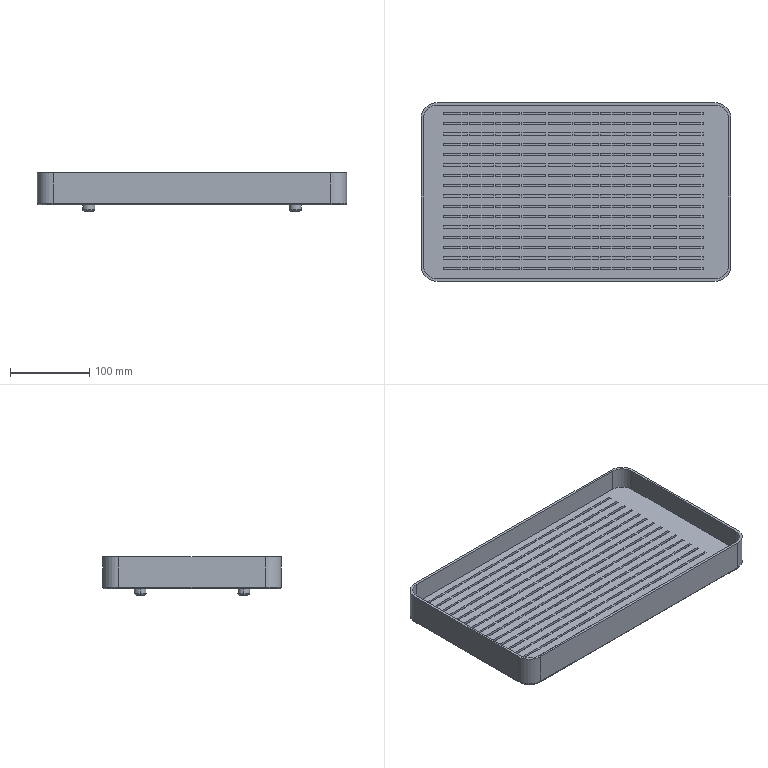Part | SolidWorks | features AEMSimFeature 1 | 2 solids | 822 faces | box 390 x 225 x 48 mm | volume 613615 mm3 | plane 786 | cylinder 24 | torus 12 | commonest cylinder face diameters 15 x8 34 x8 4 x4 40 x4